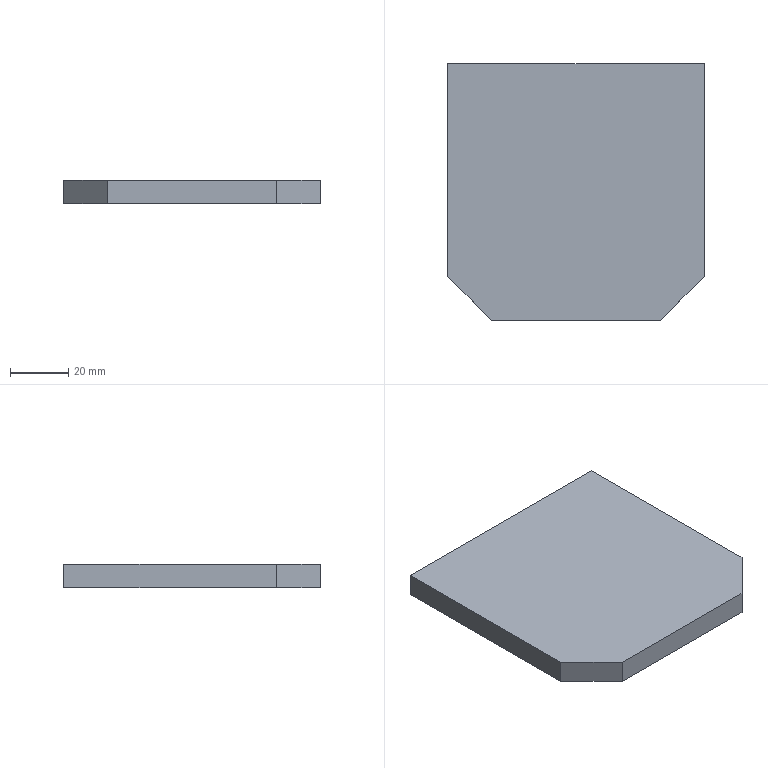Part | STEP file | _50001 | 1 solid | 8 faces | box 88 x 88 x 8 mm | volume 60152 mm3 | plane 8
STEP:
#1=CARTESIAN_POINT('',(-44.,-79.,-725.));
#2=VERTEX_POINT('',#1);
#3=CARTESIAN_POINT('',(-44.,-79.,-717.));
#4=VERTEX_POINT('',#3);
#5=CARTESIAN_POINT('',(-44.,-79.,-725.));
#6=DIRECTION('',(0.,0.,1.));
#7=VECTOR('',#6,1000.);
#8=LINE('',#5,#7);
#9=EDGE_CURVE('',#2,#4,#8,.T.);
#10=ORIENTED_EDGE('',*,*,#9,.T.);
#11=CARTESIAN_POINT('',(-44.,-6.,-717.));
#12=VERTEX_POINT('',#11);
#13=CARTESIAN_POINT('',(-44.,-6.,-717.));
#14=DIRECTION('',(0.,-1.,0.));
#15=VECTOR('',#14,1000.);
#16=LINE('',#13,#15);
#17=EDGE_CURVE('',#12,#4,#16,.T.);
#18=ORIENTED_EDGE('',*,*,#17,.F.);
#19=CARTESIAN_POINT('',(-44.,-6.,-725.));
#20=VERTEX_POINT('',#19);
#21=CARTESIAN_POINT('',(-44.,-6.,-725.));
#22=DIRECTION('',(0.,0.,1.));
#23=VECTOR('',#22,1000.);
#24=LINE('',#21,#23);
#25=EDGE_CURVE('',#20,#12,#24,.T.);
#26=ORIENTED_EDGE('',*,*,#25,.F.);
#27=CARTESIAN_POINT('',(-44.,-79.,-725.));
#28=DIRECTION('',(0.,1.,0.));
#29=VECTOR('',#28,1000.);
#30=LINE('',#27,#29);
#31=EDGE_CURVE('',#2,#20,#30,.T.);
#32=ORIENTED_EDGE('',*,*,#31,.F.);
#33=EDGE_LOOP('',(#10,#18,#26,#32));
#34=FACE_OUTER_BOUND('',#33,.T.);
#35=CARTESIAN_POINT('',(-44.,-23.,-717.));
#36=DIRECTION('',(-1.,0.,0.));
#37=DIRECTION('',(0.,0.,1.));
#38=AXIS2_PLACEMENT_3D('',#35,#36,#37);
#39=PLANE('',#38);
#40=ADVANCED_FACE('',(#34),#39,.T.);
#41=CARTESIAN_POINT('',(-29.,-94.,-725.));
#42=VERTEX_POINT('',#41);
#43=CARTESIAN_POINT('',(-29.,-94.,-717.));
#44=VERTEX_POINT('',#43);
#45=CARTESIAN_POINT('',(-29.,-94.,-725.));
#46=DIRECTION('',(0.,0.,1.));
#47=VECTOR('',#46,1000.);
#48=LINE('',#45,#47);
#49=EDGE_CURVE('',#42,#44,#48,.T.);
#50=ORIENTED_EDGE('',*,*,#49,.T.);
#51=CARTESIAN_POINT('',(-44.,-79.,-717.));
#52=DIRECTION('',(0.7071,-0.7071,0.));
#53=VECTOR('',#52,1000.);
#54=LINE('',#51,#53);
#55=EDGE_CURVE('',#4,#44,#54,.T.);
#56=ORIENTED_EDGE('',*,*,#55,.F.);
#57=ORIENTED_EDGE('',*,*,#9,.F.);
#58=CARTESIAN_POINT('',(-29.,-94.,-725.));
#59=DIRECTION('',(-0.7071,0.7071,0.));
#60=VECTOR('',#59,1000.);
#61=LINE('',#58,#60);
#62=EDGE_CURVE('',#42,#2,#61,.T.);
#63=ORIENTED_EDGE('',*,*,#62,.F.);
#64=EDGE_LOOP('',(#50,#56,#57,#63));
#65=FACE_OUTER_BOUND('',#64,.T.);
#66=CARTESIAN_POINT('',(-44.,-79.,-717.));
#67=DIRECTION('',(-0.7071,-0.7071,0.));
#68=DIRECTION('',(-0.7071,0.7071,0.));
#69=AXIS2_PLACEMENT_3D('',#66,#67,#68);
#70=PLANE('',#69);
#71=ADVANCED_FACE('',(#65),#70,.T.);
#72=CARTESIAN_POINT('',(29.,-94.,-725.));
#73=VERTEX_POINT('',#72);
#74=CARTESIAN_POINT('',(29.,-94.,-717.));
#75=VERTEX_POINT('',#74);
#76=CARTESIAN_POINT('',(29.,-94.,-725.));
#77=DIRECTION('',(0.,0.,1.));
#78=VECTOR('',#77,1000.);
#79=LINE('',#76,#78);
#80=EDGE_CURVE('',#73,#75,#79,.T.);
#81=ORIENTED_EDGE('',*,*,#80,.T.);
#82=CARTESIAN_POINT('',(-29.,-94.,-717.));
#83=DIRECTION('',(1.,0.,0.));
#84=VECTOR('',#83,1000.);
#85=LINE('',#82,#84);
#86=EDGE_CURVE('',#44,#75,#85,.T.);
#87=ORIENTED_EDGE('',*,*,#86,.F.);
#88=ORIENTED_EDGE('',*,*,#49,.F.);
#89=CARTESIAN_POINT('',(-29.,-94.,-725.));
#90=DIRECTION('',(1.,0.,0.));
#91=VECTOR('',#90,1000.);
#92=LINE('',#89,#91);
#93=EDGE_CURVE('',#42,#73,#92,.T.);
#94=ORIENTED_EDGE('',*,*,#93,.T.);
#95=EDGE_LOOP('',(#81,#87,#88,#94));
#96=FACE_OUTER_BOUND('',#95,.T.);
#97=CARTESIAN_POINT('',(-29.,-94.,-717.));
#98=DIRECTION('',(0.,-1.,0.));
#99=DIRECTION('',(0.,0.,-1.));
#100=AXIS2_PLACEMENT_3D('',#97,#98,#99);
#101=PLANE('',#100);
#102=ADVANCED_FACE('',(#96),#101,.T.);
#103=CARTESIAN_POINT('',(44.,-79.,-725.));
#104=VERTEX_POINT('',#103);
#105=CARTESIAN_POINT('',(44.,-79.,-717.));
#106=VERTEX_POINT('',#105);
#107=CARTESIAN_POINT('',(44.,-79.,-725.));
#108=DIRECTION('',(0.,0.,1.));
#109=VECTOR('',#108,1000.);
#110=LINE('',#107,#109);
#111=EDGE_CURVE('',#104,#106,#110,.T.);
#112=ORIENTED_EDGE('',*,*,#111,.T.);
#113=CARTESIAN_POINT('',(29.,-94.,-717.));
#114=DIRECTION('',(0.7071,0.7071,0.));
#115=VECTOR('',#114,1000.);
#116=LINE('',#113,#115);
#117=EDGE_CURVE('',#75,#106,#116,.T.);
#118=ORIENTED_EDGE('',*,*,#117,.F.);
#119=ORIENTED_EDGE('',*,*,#80,.F.);
#120=CARTESIAN_POINT('',(44.,-79.,-725.));
#121=DIRECTION('',(-0.7071,-0.7071,0.));
#122=VECTOR('',#121,1000.);
#123=LINE('',#120,#122);
#124=EDGE_CURVE('',#104,#73,#123,.T.);
#125=ORIENTED_EDGE('',*,*,#124,.F.);
#126=EDGE_LOOP('',(#112,#118,#119,#125));
#127=FACE_OUTER_BOUND('',#126,.T.);
#128=CARTESIAN_POINT('',(29.,-94.,-717.));
#129=DIRECTION('',(0.7071,-0.7071,0.));
#130=DIRECTION('',(0.,0.,-1.));
#131=AXIS2_PLACEMENT_3D('',#128,#129,#130);
#132=PLANE('',#131);
#133=ADVANCED_FACE('',(#127),#132,.T.);
#134=ORIENTED_EDGE('',*,*,#17,.T.);
#135=ORIENTED_EDGE('',*,*,#55,.T.);
#136=ORIENTED_EDGE('',*,*,#86,.T.);
#137=ORIENTED_EDGE('',*,*,#117,.T.);
#138=CARTESIAN_POINT('',(44.,-6.,-717.));
#139=VERTEX_POINT('',#138);
#140=CARTESIAN_POINT('',(44.,-6.,-717.));
#141=DIRECTION('',(0.,-1.,0.));
#142=VECTOR('',#141,1000.);
#143=LINE('',#140,#142);
#144=EDGE_CURVE('',#139,#106,#143,.T.);
#145=ORIENTED_EDGE('',*,*,#144,.F.);
#146=CARTESIAN_POINT('',(44.,-6.,-717.));
#147=DIRECTION('',(-1.,0.,0.));
#148=VECTOR('',#147,1000.);
#149=LINE('',#146,#148);
#150=EDGE_CURVE('',#139,#12,#149,.T.);
#151=ORIENTED_EDGE('',*,*,#150,.T.);
#152=EDGE_LOOP('',(#134,#135,#136,#137,#145,#151));
#153=FACE_OUTER_BOUND('',#152,.T.);
#154=CARTESIAN_POINT('',(0.,0.,-717.));
#155=DIRECTION('',(0.,0.,1.));
#156=DIRECTION('',(1.,0.,0.));
#157=AXIS2_PLACEMENT_3D('',#154,#155,#156);
#158=PLANE('',#157);
#159=ADVANCED_FACE('',(#153),#158,.T.);
#160=ORIENTED_EDGE('',*,*,#111,.F.);
#161=CARTESIAN_POINT('',(44.,-6.,-725.));
#162=VERTEX_POINT('',#161);
#163=CARTESIAN_POINT('',(44.,-6.,-725.));
#164=DIRECTION('',(0.,-1.,0.));
#165=VECTOR('',#164,1000.);
#166=LINE('',#163,#165);
#167=EDGE_CURVE('',#162,#104,#166,.T.);
#168=ORIENTED_EDGE('',*,*,#167,.F.);
#169=CARTESIAN_POINT('',(44.,-6.,-725.));
#170=DIRECTION('',(0.,0.,1.));
#171=VECTOR('',#170,1000.);
#172=LINE('',#169,#171);
#173=EDGE_CURVE('',#162,#139,#172,.T.);
#174=ORIENTED_EDGE('',*,*,#173,.T.);
#175=ORIENTED_EDGE('',*,*,#144,.T.);
#176=EDGE_LOOP('',(#160,#168,#174,#175));
#177=FACE_OUTER_BOUND('',#176,.T.);
#178=CARTESIAN_POINT('',(44.,-79.,-717.));
#179=DIRECTION('',(1.,0.,0.));
#180=DIRECTION('',(0.,1.,0.));
#181=AXIS2_PLACEMENT_3D('',#178,#179,#180);
#182=PLANE('',#181);
#183=ADVANCED_FACE('',(#177),#182,.T.);
#184=ORIENTED_EDGE('',*,*,#124,.T.);
#185=ORIENTED_EDGE('',*,*,#93,.F.);
#186=ORIENTED_EDGE('',*,*,#62,.T.);
#187=ORIENTED_EDGE('',*,*,#31,.T.);
#188=CARTESIAN_POINT('',(-44.,-6.,-725.));
#189=DIRECTION('',(1.,0.,0.));
#190=VECTOR('',#189,1000.);
#191=LINE('',#188,#190);
#192=EDGE_CURVE('',#20,#162,#191,.T.);
#193=ORIENTED_EDGE('',*,*,#192,.T.);
#194=ORIENTED_EDGE('',*,*,#167,.T.);
#195=EDGE_LOOP('',(#184,#185,#186,#187,#193,#194));
#196=FACE_OUTER_BOUND('',#195,.T.);
#197=CARTESIAN_POINT('',(0.,0.,-725.));
#198=DIRECTION('',(0.,0.,1.));
#199=DIRECTION('',(1.,0.,0.));
#200=AXIS2_PLACEMENT_3D('',#197,#198,#199);
#201=PLANE('',#200);
#202=ADVANCED_FACE('',(#196),#201,.F.);
#203=ORIENTED_EDGE('',*,*,#25,.T.);
#204=ORIENTED_EDGE('',*,*,#150,.F.);
#205=ORIENTED_EDGE('',*,*,#173,.F.);
#206=ORIENTED_EDGE('',*,*,#192,.F.);
#207=EDGE_LOOP('',(#203,#204,#205,#206));
#208=FACE_OUTER_BOUND('',#207,.T.);
#209=CARTESIAN_POINT('',(29.,-6.,-717.));
#210=DIRECTION('',(0.,1.,0.));
#211=DIRECTION('',(1.,0.,0.));
#212=AXIS2_PLACEMENT_3D('',#209,#210,#211);
#213=PLANE('',#212);
#214=ADVANCED_FACE('',(#208),#213,.T.);
#215=CLOSED_SHELL('',(#40,#71,#102,#133,#159,#183,#202,#214));
#216=MANIFOLD_SOLID_BREP('',#215);
#217=CARTESIAN_POINT('',(0.,0.,0.));
#218=DIRECTION('',(0.,0.,1.));
#219=DIRECTION('',(1.,0.,0.));
#220=AXIS2_PLACEMENT_3D('',#217,#218,#219);
#221=(LENGTH_UNIT()NAMED_UNIT(*)SI_UNIT(.MILLI.,.METRE.));
#222=UNCERTAINTY_MEASURE_WITH_UNIT(LENGTH_MEASURE(0.00001),#221,'','');
#223=(NAMED_UNIT(*)PLANE_ANGLE_UNIT()SI_UNIT($,.RADIAN.));
#224=(NAMED_UNIT(*)SI_UNIT($,.STERADIAN.)SOLID_ANGLE_UNIT());
#225=(GEOMETRIC_REPRESENTATION_CONTEXT(3)GLOBAL_UNCERTAINTY_ASSIGNED_CONTEXT((#222))GLOBAL_UNIT_ASSIGNED_CONTEXT((#221,#223,#224))REPRESENTATION_CONTEXT('',''));
#226=ADVANCED_BREP_SHAPE_REPRESENTATION('',(#216,#220),#225);